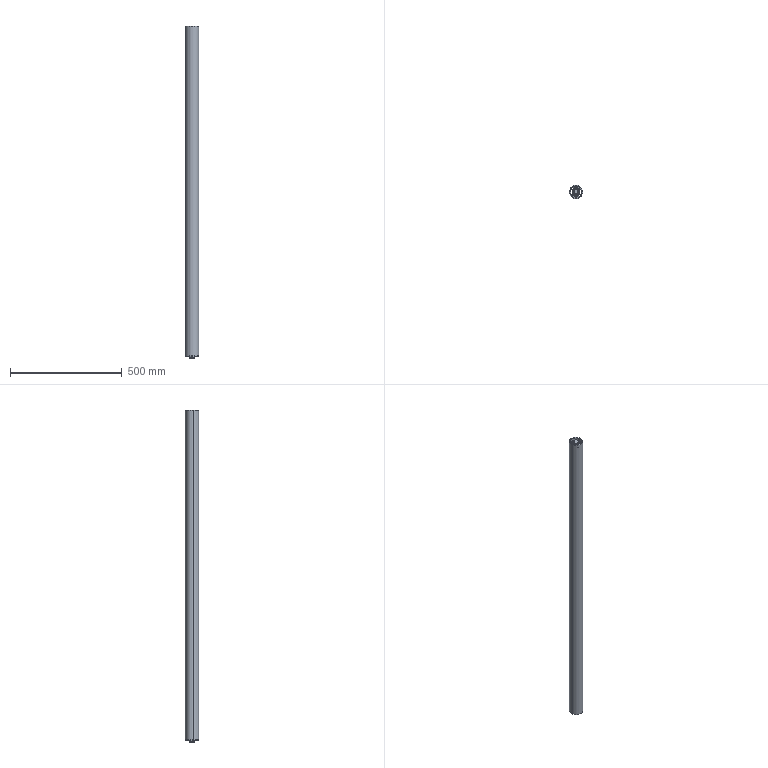Part | SolidWorks | 4 solids | 260 faces | box 60 x 60 x 1489 mm | volume 2237617 mm3 | torus 124 | sphere 68 | cylinder 42 | plane 18 | cone 8 | commonest cylinder face diameters 23 x8 29 x8 25 x6 17 x4 23.9 x4 35 x4